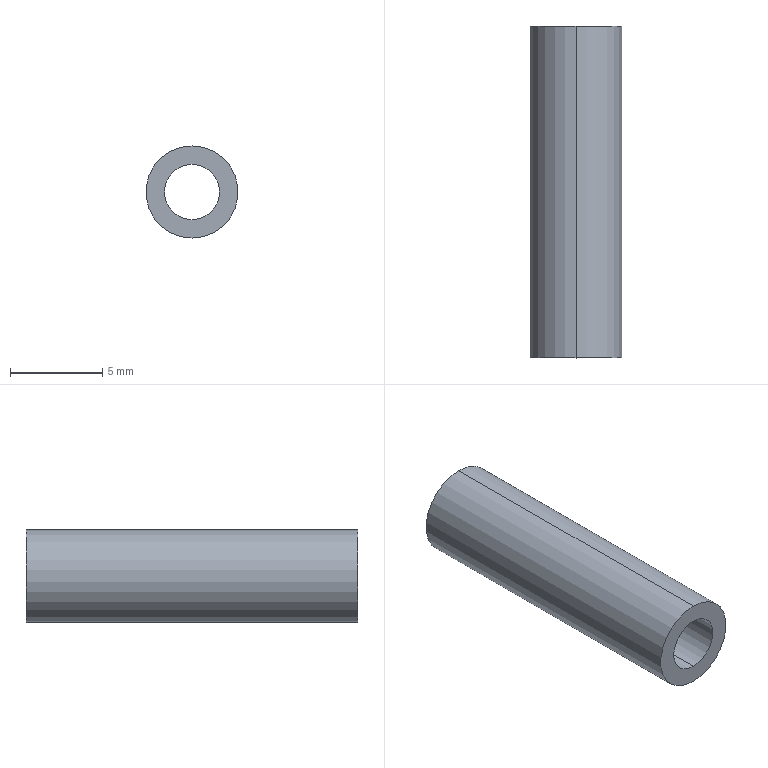Part | SolidWorks | features Extrusion 1 | 1 solid | 6 faces | box 5 x 18 x 5 mm | volume 226.195 mm3 | cylinder 4 | plane 2 | commonest cylinder face diameters 3 x2 5 x2
STEP:
#1=CARTESIAN_POINT('',(0.,18.,-1.5));
#2=VERTEX_POINT('',#1);
#3=CARTESIAN_POINT('',(0.,18.,1.5));
#4=VERTEX_POINT('',#3);
#5=CARTESIAN_POINT('',(0.,18.,0.));
#6=DIRECTION('',(0.,1.,0.));
#7=DIRECTION('',(0.,0.,1.));
#8=AXIS2_PLACEMENT_3D('',#5,#6,#7);
#9=CIRCLE('',#8,1.5);
#10=EDGE_CURVE('',#2,#4,#9,.T.);
#11=ORIENTED_EDGE('',*,*,#10,.T.);
#12=CARTESIAN_POINT('',(0.,0.,1.5));
#13=VERTEX_POINT('',#12);
#14=CARTESIAN_POINT('',(0.,18.,1.5));
#15=DIRECTION('',(0.,-1.,0.));
#16=VECTOR('',#15,1000.);
#17=LINE('',#14,#16);
#18=EDGE_CURVE('',#4,#13,#17,.T.);
#19=ORIENTED_EDGE('',*,*,#18,.T.);
#20=CARTESIAN_POINT('',(0.,0.,-1.5));
#21=VERTEX_POINT('',#20);
#22=CARTESIAN_POINT('',(0.,0.,0.));
#23=DIRECTION('',(0.,1.,0.));
#24=DIRECTION('',(0.,0.,1.));
#25=AXIS2_PLACEMENT_3D('',#22,#23,#24);
#26=CIRCLE('',#25,1.5);
#27=EDGE_CURVE('',#21,#13,#26,.T.);
#28=ORIENTED_EDGE('',*,*,#27,.F.);
#29=CARTESIAN_POINT('',(0.,18.,-1.5));
#30=DIRECTION('',(0.,-1.,0.));
#31=VECTOR('',#30,1000.);
#32=LINE('',#29,#31);
#33=EDGE_CURVE('',#2,#21,#32,.T.);
#34=ORIENTED_EDGE('',*,*,#33,.F.);
#35=EDGE_LOOP('',(#11,#19,#28,#34));
#36=FACE_OUTER_BOUND('',#35,.T.);
#37=CARTESIAN_POINT('',(0.,18.,0.));
#38=DIRECTION('',(0.,-1.,0.));
#39=DIRECTION('',(0.,0.,-1.));
#40=AXIS2_PLACEMENT_3D('',#37,#38,#39);
#41=CYLINDRICAL_SURFACE('',#40,1.5);
#42=ADVANCED_FACE('',(#36),#41,.F.);
#43=CARTESIAN_POINT('',(0.,18.,2.5));
#44=VERTEX_POINT('',#43);
#45=CARTESIAN_POINT('',(0.,18.,-2.5));
#46=VERTEX_POINT('',#45);
#47=CARTESIAN_POINT('',(0.,18.,0.));
#48=DIRECTION('',(0.,1.,0.));
#49=DIRECTION('',(0.,0.,1.));
#50=AXIS2_PLACEMENT_3D('',#47,#48,#49);
#51=CIRCLE('',#50,2.5);
#52=EDGE_CURVE('',#44,#46,#51,.T.);
#53=ORIENTED_EDGE('',*,*,#52,.F.);
#54=CARTESIAN_POINT('',(0.,0.,2.5));
#55=VERTEX_POINT('',#54);
#56=CARTESIAN_POINT('',(0.,18.,2.5));
#57=DIRECTION('',(0.,-1.,0.));
#58=VECTOR('',#57,1000.);
#59=LINE('',#56,#58);
#60=EDGE_CURVE('',#44,#55,#59,.T.);
#61=ORIENTED_EDGE('',*,*,#60,.T.);
#62=CARTESIAN_POINT('',(0.,0.,-2.5));
#63=VERTEX_POINT('',#62);
#64=CARTESIAN_POINT('',(0.,0.,0.));
#65=DIRECTION('',(0.,1.,0.));
#66=DIRECTION('',(0.,0.,1.));
#67=AXIS2_PLACEMENT_3D('',#64,#65,#66);
#68=CIRCLE('',#67,2.5);
#69=EDGE_CURVE('',#55,#63,#68,.T.);
#70=ORIENTED_EDGE('',*,*,#69,.T.);
#71=CARTESIAN_POINT('',(0.,18.,-2.5));
#72=DIRECTION('',(0.,-1.,0.));
#73=VECTOR('',#72,1000.);
#74=LINE('',#71,#73);
#75=EDGE_CURVE('',#46,#63,#74,.T.);
#76=ORIENTED_EDGE('',*,*,#75,.F.);
#77=EDGE_LOOP('',(#53,#61,#70,#76));
#78=FACE_OUTER_BOUND('',#77,.T.);
#79=CARTESIAN_POINT('',(0.,18.,0.));
#80=DIRECTION('',(0.,-1.,0.));
#81=DIRECTION('',(0.,0.,-1.));
#82=AXIS2_PLACEMENT_3D('',#79,#80,#81);
#83=CYLINDRICAL_SURFACE('',#82,2.5);
#84=ADVANCED_FACE('',(#78),#83,.T.);
#85=CARTESIAN_POINT('',(0.,18.,0.));
#86=DIRECTION('',(0.,1.,0.));
#87=DIRECTION('',(0.,0.,1.));
#88=AXIS2_PLACEMENT_3D('',#85,#86,#87);
#89=CIRCLE('',#88,2.5);
#90=EDGE_CURVE('',#46,#44,#89,.T.);
#91=ORIENTED_EDGE('',*,*,#90,.T.);
#92=ORIENTED_EDGE('',*,*,#52,.T.);
#93=EDGE_LOOP('',(#91,#92));
#94=FACE_OUTER_BOUND('',#93,.T.);
#95=ORIENTED_EDGE('',*,*,#10,.F.);
#96=CARTESIAN_POINT('',(0.,18.,0.));
#97=DIRECTION('',(0.,1.,0.));
#98=DIRECTION('',(0.,0.,1.));
#99=AXIS2_PLACEMENT_3D('',#96,#97,#98);
#100=CIRCLE('',#99,1.5);
#101=EDGE_CURVE('',#4,#2,#100,.T.);
#102=ORIENTED_EDGE('',*,*,#101,.F.);
#103=EDGE_LOOP('',(#95,#102));
#104=FACE_BOUND('',#103,.T.);
#105=CARTESIAN_POINT('',(0.,18.,0.));
#106=DIRECTION('',(0.,1.,0.));
#107=DIRECTION('',(0.,0.,1.));
#108=AXIS2_PLACEMENT_3D('',#105,#106,#107);
#109=PLANE('',#108);
#110=ADVANCED_FACE('',(#94,#104),#109,.T.);
#111=CARTESIAN_POINT('',(0.,0.,0.));
#112=DIRECTION('',(0.,1.,0.));
#113=DIRECTION('',(0.,0.,1.));
#114=AXIS2_PLACEMENT_3D('',#111,#112,#113);
#115=CIRCLE('',#114,2.5);
#116=EDGE_CURVE('',#63,#55,#115,.T.);
#117=ORIENTED_EDGE('',*,*,#116,.F.);
#118=ORIENTED_EDGE('',*,*,#69,.F.);
#119=EDGE_LOOP('',(#117,#118));
#120=FACE_OUTER_BOUND('',#119,.T.);
#121=ORIENTED_EDGE('',*,*,#27,.T.);
#122=CARTESIAN_POINT('',(0.,0.,0.));
#123=DIRECTION('',(0.,1.,0.));
#124=DIRECTION('',(0.,0.,1.));
#125=AXIS2_PLACEMENT_3D('',#122,#123,#124);
#126=CIRCLE('',#125,1.5);
#127=EDGE_CURVE('',#13,#21,#126,.T.);
#128=ORIENTED_EDGE('',*,*,#127,.T.);
#129=EDGE_LOOP('',(#121,#128));
#130=FACE_BOUND('',#129,.T.);
#131=CARTESIAN_POINT('',(0.,0.,0.));
#132=DIRECTION('',(0.,1.,0.));
#133=DIRECTION('',(0.,0.,1.));
#134=AXIS2_PLACEMENT_3D('',#131,#132,#133);
#135=PLANE('',#134);
#136=ADVANCED_FACE('',(#120,#130),#135,.F.);
#137=ORIENTED_EDGE('',*,*,#60,.F.);
#138=ORIENTED_EDGE('',*,*,#90,.F.);
#139=ORIENTED_EDGE('',*,*,#75,.T.);
#140=ORIENTED_EDGE('',*,*,#116,.T.);
#141=EDGE_LOOP('',(#137,#138,#139,#140));
#142=FACE_OUTER_BOUND('',#141,.T.);
#143=CARTESIAN_POINT('',(0.,18.,0.));
#144=DIRECTION('',(0.,-1.,0.));
#145=DIRECTION('',(0.,0.,-1.));
#146=AXIS2_PLACEMENT_3D('',#143,#144,#145);
#147=CYLINDRICAL_SURFACE('',#146,2.5);
#148=ADVANCED_FACE('',(#142),#147,.T.);
#149=ORIENTED_EDGE('',*,*,#18,.F.);
#150=ORIENTED_EDGE('',*,*,#101,.T.);
#151=ORIENTED_EDGE('',*,*,#33,.T.);
#152=ORIENTED_EDGE('',*,*,#127,.F.);
#153=EDGE_LOOP('',(#149,#150,#151,#152));
#154=FACE_OUTER_BOUND('',#153,.T.);
#155=CARTESIAN_POINT('',(0.,18.,0.));
#156=DIRECTION('',(0.,-1.,0.));
#157=DIRECTION('',(0.,0.,-1.));
#158=AXIS2_PLACEMENT_3D('',#155,#156,#157);
#159=CYLINDRICAL_SURFACE('',#158,1.5);
#160=ADVANCED_FACE('',(#154),#159,.F.);
#161=CLOSED_SHELL('',(#42,#84,#110,#136,#148,#160));
#162=MANIFOLD_SOLID_BREP('',#161);
#163=CARTESIAN_POINT('',(0.,0.,0.));
#164=DIRECTION('',(0.,0.,1.));
#165=DIRECTION('',(1.,0.,0.));
#166=AXIS2_PLACEMENT_3D('',#163,#164,#165);
#167=(LENGTH_UNIT()NAMED_UNIT(*)SI_UNIT(.MILLI.,.METRE.));
#168=UNCERTAINTY_MEASURE_WITH_UNIT(LENGTH_MEASURE(0.00001),#167,'','');
#169=(NAMED_UNIT(*)PLANE_ANGLE_UNIT()SI_UNIT($,.RADIAN.));
#170=(NAMED_UNIT(*)SI_UNIT($,.STERADIAN.)SOLID_ANGLE_UNIT());
#171=(GEOMETRIC_REPRESENTATION_CONTEXT(3)GLOBAL_UNCERTAINTY_ASSIGNED_CONTEXT((#168))GLOBAL_UNIT_ASSIGNED_CONTEXT((#167,#169,#170))REPRESENTATION_CONTEXT('',''));
#172=ADVANCED_BREP_SHAPE_REPRESENTATION('',(#162,#166),#171);